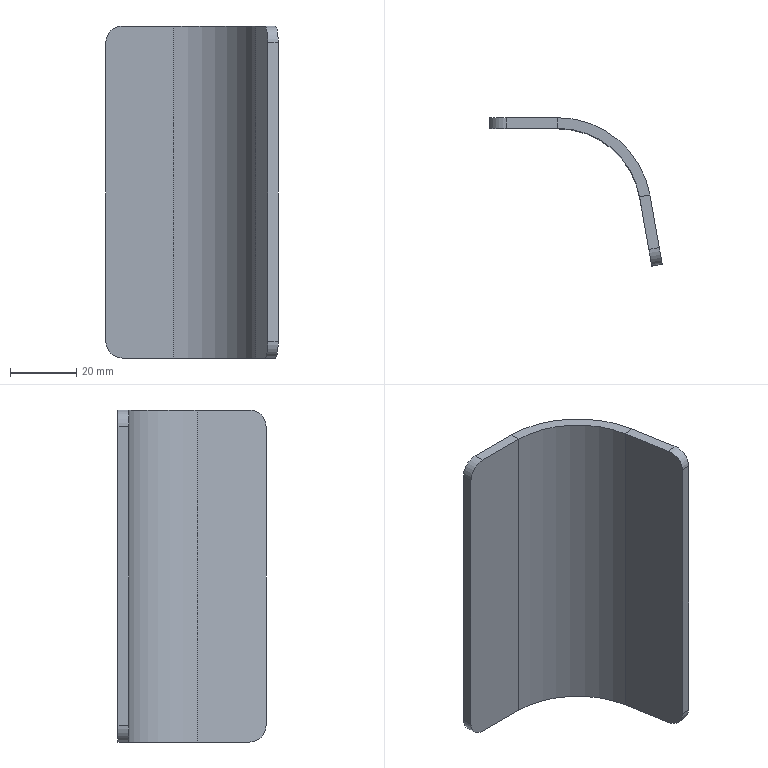Part | SolidWorks | features Fillet 1, FlatPattern 1, SMBaseFlange 1, SheetMetal 1 | 1 solid | 18 faces | box 51.9 x 44.589 x 100 mm | volume 25102 mm3 | plane 12 | cylinder 6 | commonest cylinder face diameters 10 x4 50 x1 56.4 x1
STEP:
#1=CARTESIAN_POINT('',(4.116,-23.293,50.));
#2=VERTEX_POINT('',#1);
#3=CARTESIAN_POINT('',(0.9645,-23.85,50.));
#4=VERTEX_POINT('',#3);
#5=CARTESIAN_POINT('',(4.116,-23.293,50.));
#6=DIRECTION('',(-0.9847,-0.174,0.));
#7=VECTOR('',#6,1000.);
#8=LINE('',#5,#7);
#9=EDGE_CURVE('',#2,#4,#8,.T.);
#10=ORIENTED_EDGE('',*,*,#9,.F.);
#11=CARTESIAN_POINT('',(-23.654,0.,50.));
#12=VERTEX_POINT('',#11);
#13=CARTESIAN_POINT('',(-23.654,-28.2,50.));
#14=DIRECTION('',(0.,0.,-1.));
#15=DIRECTION('',(1.,0.,0.));
#16=AXIS2_PLACEMENT_3D('',#13,#14,#15);
#17=CIRCLE('',#16,28.2);
#18=EDGE_CURVE('',#12,#2,#17,.T.);
#19=ORIENTED_EDGE('',*,*,#18,.F.);
#20=CARTESIAN_POINT('',(-23.654,-3.2,50.));
#21=VERTEX_POINT('',#20);
#22=CARTESIAN_POINT('',(-23.654,-3.2,50.));
#23=DIRECTION('',(0.,1.,0.));
#24=VECTOR('',#23,1000.);
#25=LINE('',#22,#24);
#26=EDGE_CURVE('',#21,#12,#25,.T.);
#27=ORIENTED_EDGE('',*,*,#26,.F.);
#28=CARTESIAN_POINT('',(-23.654,-28.2,50.));
#29=DIRECTION('',(0.,0.,-1.));
#30=DIRECTION('',(1.,0.,0.));
#31=AXIS2_PLACEMENT_3D('',#28,#29,#30);
#32=CIRCLE('',#31,25.);
#33=EDGE_CURVE('',#21,#4,#32,.T.);
#34=ORIENTED_EDGE('',*,*,#33,.T.);
#35=EDGE_LOOP('',(#10,#19,#27,#34));
#36=FACE_OUTER_BOUND('',#35,.T.);
#37=CARTESIAN_POINT('',(4.116,-23.293,50.));
#38=DIRECTION('',(0.,0.,1.));
#39=DIRECTION('',(1.,0.,0.));
#40=AXIS2_PLACEMENT_3D('',#37,#38,#39);
#41=PLANE('',#40);
#42=ADVANCED_FACE('',(#36),#41,.T.);
#43=CARTESIAN_POINT('',(3.759,-39.666,50.));
#44=VERTEX_POINT('',#43);
#45=CARTESIAN_POINT('',(-3.151,-0.5568,50.));
#46=DIRECTION('',(0.174,-0.9847,0.));
#47=VECTOR('',#46,1000.);
#48=LINE('',#45,#47);
#49=EDGE_CURVE('',#4,#44,#48,.T.);
#50=ORIENTED_EDGE('',*,*,#49,.T.);
#51=CARTESIAN_POINT('',(6.91,-39.109,50.));
#52=VERTEX_POINT('',#51);
#53=CARTESIAN_POINT('',(-16.576,-43.259,50.));
#54=DIRECTION('',(0.9847,0.174,0.));
#55=VECTOR('',#54,1000.);
#56=LINE('',#53,#55);
#57=EDGE_CURVE('',#44,#52,#56,.T.);
#58=ORIENTED_EDGE('',*,*,#57,.T.);
#59=CARTESIAN_POINT('',(0.,0.,50.));
#60=DIRECTION('',(0.174,-0.9847,0.));
#61=VECTOR('',#60,1000.);
#62=LINE('',#59,#61);
#63=EDGE_CURVE('',#2,#52,#62,.T.);
#64=ORIENTED_EDGE('',*,*,#63,.F.);
#65=ORIENTED_EDGE('',*,*,#9,.T.);
#66=EDGE_LOOP('',(#50,#58,#64,#65));
#67=FACE_OUTER_BOUND('',#66,.T.);
#68=CARTESIAN_POINT('',(-23.654,-3.2,50.));
#69=DIRECTION('',(0.,0.,1.));
#70=DIRECTION('',(1.,0.,0.));
#71=AXIS2_PLACEMENT_3D('',#68,#69,#70);
#72=PLANE('',#71);
#73=ADVANCED_FACE('',(#67),#72,.T.);
#74=CARTESIAN_POINT('',(-23.654,0.,-50.));
#75=VERTEX_POINT('',#74);
#76=CARTESIAN_POINT('',(-23.654,-3.2,-50.));
#77=VERTEX_POINT('',#76);
#78=CARTESIAN_POINT('',(-23.654,0.,-50.));
#79=DIRECTION('',(0.,-1.,0.));
#80=VECTOR('',#79,1000.);
#81=LINE('',#78,#80);
#82=EDGE_CURVE('',#75,#77,#81,.T.);
#83=ORIENTED_EDGE('',*,*,#82,.F.);
#84=CARTESIAN_POINT('',(4.116,-23.293,-50.));
#85=VERTEX_POINT('',#84);
#86=CARTESIAN_POINT('',(-23.654,-28.2,-50.));
#87=DIRECTION('',(0.,0.,-1.));
#88=DIRECTION('',(1.,0.,0.));
#89=AXIS2_PLACEMENT_3D('',#86,#87,#88);
#90=CIRCLE('',#89,28.2);
#91=EDGE_CURVE('',#75,#85,#90,.T.);
#92=ORIENTED_EDGE('',*,*,#91,.T.);
#93=CARTESIAN_POINT('',(0.9645,-23.85,-50.));
#94=VERTEX_POINT('',#93);
#95=CARTESIAN_POINT('',(0.9645,-23.85,-50.));
#96=DIRECTION('',(0.9847,0.174,0.));
#97=VECTOR('',#96,1000.);
#98=LINE('',#95,#97);
#99=EDGE_CURVE('',#94,#85,#98,.T.);
#100=ORIENTED_EDGE('',*,*,#99,.F.);
#101=CARTESIAN_POINT('',(-23.654,-28.2,-50.));
#102=DIRECTION('',(0.,0.,-1.));
#103=DIRECTION('',(1.,0.,0.));
#104=AXIS2_PLACEMENT_3D('',#101,#102,#103);
#105=CIRCLE('',#104,25.);
#106=EDGE_CURVE('',#77,#94,#105,.T.);
#107=ORIENTED_EDGE('',*,*,#106,.F.);
#108=EDGE_LOOP('',(#83,#92,#100,#107));
#109=FACE_OUTER_BOUND('',#108,.T.);
#110=CARTESIAN_POINT('',(-23.654,0.,-50.));
#111=DIRECTION('',(0.,0.,-1.));
#112=DIRECTION('',(-1.,0.,0.));
#113=AXIS2_PLACEMENT_3D('',#110,#111,#112);
#114=PLANE('',#113);
#115=ADVANCED_FACE('',(#109),#114,.T.);
#116=CARTESIAN_POINT('',(-39.12,-3.2,-50.));
#117=VERTEX_POINT('',#116);
#118=CARTESIAN_POINT('',(0.,-3.2,-50.));
#119=DIRECTION('',(1.,0.,0.));
#120=VECTOR('',#119,1000.);
#121=LINE('',#118,#120);
#122=EDGE_CURVE('',#117,#77,#121,.T.);
#123=ORIENTED_EDGE('',*,*,#122,.F.);
#124=CARTESIAN_POINT('',(-39.12,0.,-50.));
#125=VERTEX_POINT('',#124);
#126=CARTESIAN_POINT('',(-39.12,-23.85,-50.));
#127=DIRECTION('',(0.,1.,0.));
#128=VECTOR('',#127,1000.);
#129=LINE('',#126,#128);
#130=EDGE_CURVE('',#117,#125,#129,.T.);
#131=ORIENTED_EDGE('',*,*,#130,.T.);
#132=CARTESIAN_POINT('',(0.,0.,-50.));
#133=DIRECTION('',(1.,0.,0.));
#134=VECTOR('',#133,1000.);
#135=LINE('',#132,#134);
#136=EDGE_CURVE('',#125,#75,#135,.T.);
#137=ORIENTED_EDGE('',*,*,#136,.T.);
#138=ORIENTED_EDGE('',*,*,#82,.T.);
#139=EDGE_LOOP('',(#123,#131,#137,#138));
#140=FACE_OUTER_BOUND('',#139,.T.);
#141=CARTESIAN_POINT('',(0.9645,-23.85,-50.));
#142=DIRECTION('',(0.,0.,-1.));
#143=DIRECTION('',(-1.,0.,0.));
#144=AXIS2_PLACEMENT_3D('',#141,#142,#143);
#145=PLANE('',#144);
#146=ADVANCED_FACE('',(#140),#145,.T.);
#147=CARTESIAN_POINT('',(4.629,-44.589,45.));
#148=VERTEX_POINT('',#147);
#149=CARTESIAN_POINT('',(4.629,-44.589,-45.));
#150=VERTEX_POINT('',#149);
#151=CARTESIAN_POINT('',(4.629,-44.589,50.));
#152=DIRECTION('',(0.,0.,-1.));
#153=VECTOR('',#152,1000.);
#154=LINE('',#151,#153);
#155=EDGE_CURVE('',#148,#150,#154,.T.);
#156=ORIENTED_EDGE('',*,*,#155,.F.);
#157=CARTESIAN_POINT('',(3.759,-39.666,45.));
#158=DIRECTION('',(-0.9847,-0.174,0.));
#159=DIRECTION('',(-0.174,0.9847,0.));
#160=AXIS2_PLACEMENT_3D('',#157,#158,#159);
#161=CIRCLE('',#160,5.);
#162=EDGE_CURVE('',#148,#44,#161,.T.);
#163=ORIENTED_EDGE('',*,*,#162,.T.);
#164=ORIENTED_EDGE('',*,*,#49,.F.);
#165=CARTESIAN_POINT('',(0.9645,-23.85,50.));
#166=DIRECTION('',(0.,0.,-1.));
#167=VECTOR('',#166,1000.);
#168=LINE('',#165,#167);
#169=EDGE_CURVE('',#4,#94,#168,.T.);
#170=ORIENTED_EDGE('',*,*,#169,.T.);
#171=CARTESIAN_POINT('',(3.759,-39.666,-50.));
#172=VERTEX_POINT('',#171);
#173=CARTESIAN_POINT('',(-3.151,-0.5568,-50.));
#174=DIRECTION('',(0.174,-0.9847,0.));
#175=VECTOR('',#174,1000.);
#176=LINE('',#173,#175);
#177=EDGE_CURVE('',#94,#172,#176,.T.);
#178=ORIENTED_EDGE('',*,*,#177,.T.);
#179=CARTESIAN_POINT('',(3.759,-39.666,-45.));
#180=DIRECTION('',(-0.9847,-0.174,0.));
#181=DIRECTION('',(-0.174,0.9847,0.));
#182=AXIS2_PLACEMENT_3D('',#179,#180,#181);
#183=CIRCLE('',#182,5.);
#184=EDGE_CURVE('',#172,#150,#183,.T.);
#185=ORIENTED_EDGE('',*,*,#184,.T.);
#186=EDGE_LOOP('',(#156,#163,#164,#170,#178,#185));
#187=FACE_OUTER_BOUND('',#186,.T.);
#188=CARTESIAN_POINT('',(-3.151,-0.5568,50.));
#189=DIRECTION('',(0.9847,0.174,0.));
#190=DIRECTION('',(-0.174,0.9847,0.));
#191=AXIS2_PLACEMENT_3D('',#188,#189,#190);
#192=PLANE('',#191);
#193=ADVANCED_FACE('',(#187),#192,.F.);
#194=CARTESIAN_POINT('',(7.78,-44.033,45.));
#195=VERTEX_POINT('',#194);
#196=CARTESIAN_POINT('',(7.78,-44.033,-45.));
#197=VERTEX_POINT('',#196);
#198=CARTESIAN_POINT('',(7.78,-44.033,50.));
#199=DIRECTION('',(0.,0.,-1.));
#200=VECTOR('',#199,1000.);
#201=LINE('',#198,#200);
#202=EDGE_CURVE('',#195,#197,#201,.T.);
#203=ORIENTED_EDGE('',*,*,#202,.F.);
#204=CARTESIAN_POINT('',(7.78,-44.033,45.));
#205=DIRECTION('',(-0.9847,-0.174,0.));
#206=VECTOR('',#205,1000.);
#207=LINE('',#204,#206);
#208=EDGE_CURVE('',#195,#148,#207,.T.);
#209=ORIENTED_EDGE('',*,*,#208,.T.);
#210=ORIENTED_EDGE('',*,*,#155,.T.);
#211=CARTESIAN_POINT('',(7.78,-44.033,-45.));
#212=DIRECTION('',(0.9847,0.174,0.));
#213=VECTOR('',#212,1000.);
#214=LINE('',#211,#213);
#215=EDGE_CURVE('',#150,#197,#214,.T.);
#216=ORIENTED_EDGE('',*,*,#215,.T.);
#217=EDGE_LOOP('',(#203,#209,#210,#216));
#218=FACE_OUTER_BOUND('',#217,.T.);
#219=CARTESIAN_POINT('',(7.78,-44.033,50.));
#220=DIRECTION('',(0.174,-0.9847,0.));
#221=DIRECTION('',(0.9847,0.174,0.));
#222=AXIS2_PLACEMENT_3D('',#219,#220,#221);
#223=PLANE('',#222);
#224=ADVANCED_FACE('',(#218),#223,.T.);
#225=ORIENTED_EDGE('',*,*,#63,.T.);
#226=CARTESIAN_POINT('',(6.91,-39.109,45.));
#227=DIRECTION('',(0.9847,0.174,0.));
#228=DIRECTION('',(-0.174,0.9847,0.));
#229=AXIS2_PLACEMENT_3D('',#226,#227,#228);
#230=CIRCLE('',#229,5.);
#231=EDGE_CURVE('',#52,#195,#230,.T.);
#232=ORIENTED_EDGE('',*,*,#231,.T.);
#233=ORIENTED_EDGE('',*,*,#202,.T.);
#234=CARTESIAN_POINT('',(6.91,-39.109,-50.));
#235=VERTEX_POINT('',#234);
#236=CARTESIAN_POINT('',(6.91,-39.109,-45.));
#237=DIRECTION('',(0.9847,0.174,0.));
#238=DIRECTION('',(-0.174,0.9847,0.));
#239=AXIS2_PLACEMENT_3D('',#236,#237,#238);
#240=CIRCLE('',#239,5.);
#241=EDGE_CURVE('',#197,#235,#240,.T.);
#242=ORIENTED_EDGE('',*,*,#241,.T.);
#243=CARTESIAN_POINT('',(0.,0.,-50.));
#244=DIRECTION('',(0.174,-0.9847,0.));
#245=VECTOR('',#244,1000.);
#246=LINE('',#243,#245);
#247=EDGE_CURVE('',#85,#235,#246,.T.);
#248=ORIENTED_EDGE('',*,*,#247,.F.);
#249=CARTESIAN_POINT('',(4.116,-23.293,50.));
#250=DIRECTION('',(0.,0.,-1.));
#251=VECTOR('',#250,1000.);
#252=LINE('',#249,#251);
#253=EDGE_CURVE('',#2,#85,#252,.T.);
#254=ORIENTED_EDGE('',*,*,#253,.F.);
#255=EDGE_LOOP('',(#225,#232,#233,#242,#248,#254));
#256=FACE_OUTER_BOUND('',#255,.T.);
#257=CARTESIAN_POINT('',(0.,0.,50.));
#258=DIRECTION('',(0.9847,0.174,0.));
#259=DIRECTION('',(-0.174,0.9847,0.));
#260=AXIS2_PLACEMENT_3D('',#257,#258,#259);
#261=PLANE('',#260);
#262=ADVANCED_FACE('',(#256),#261,.T.);
#263=ORIENTED_EDGE('',*,*,#91,.F.);
#264=CARTESIAN_POINT('',(-23.654,0.,50.));
#265=DIRECTION('',(0.,0.,-1.));
#266=VECTOR('',#265,1000.);
#267=LINE('',#264,#266);
#268=EDGE_CURVE('',#12,#75,#267,.T.);
#269=ORIENTED_EDGE('',*,*,#268,.F.);
#270=ORIENTED_EDGE('',*,*,#18,.T.);
#271=ORIENTED_EDGE('',*,*,#253,.T.);
#272=EDGE_LOOP('',(#263,#269,#270,#271));
#273=FACE_OUTER_BOUND('',#272,.T.);
#274=CARTESIAN_POINT('',(-23.654,-28.2,50.));
#275=DIRECTION('',(0.,0.,-1.));
#276=DIRECTION('',(-1.,0.,0.));
#277=AXIS2_PLACEMENT_3D('',#274,#275,#276);
#278=CYLINDRICAL_SURFACE('',#277,28.2);
#279=ADVANCED_FACE('',(#273),#278,.T.);
#280=ORIENTED_EDGE('',*,*,#136,.F.);
#281=CARTESIAN_POINT('',(-44.12,0.,-45.));
#282=VERTEX_POINT('',#281);
#283=CARTESIAN_POINT('',(-39.12,0.,-45.));
#284=DIRECTION('',(0.,1.,0.));
#285=DIRECTION('',(-1.,0.,0.));
#286=AXIS2_PLACEMENT_3D('',#283,#284,#285);
#287=CIRCLE('',#286,5.);
#288=EDGE_CURVE('',#125,#282,#287,.T.);
#289=ORIENTED_EDGE('',*,*,#288,.T.);
#290=CARTESIAN_POINT('',(-44.12,0.,45.));
#291=VERTEX_POINT('',#290);
#292=CARTESIAN_POINT('',(-44.12,0.,50.));
#293=DIRECTION('',(0.,0.,-1.));
#294=VECTOR('',#293,1000.);
#295=LINE('',#292,#294);
#296=EDGE_CURVE('',#291,#282,#295,.T.);
#297=ORIENTED_EDGE('',*,*,#296,.F.);
#298=CARTESIAN_POINT('',(-39.12,0.,50.));
#299=VERTEX_POINT('',#298);
#300=CARTESIAN_POINT('',(-39.12,0.,45.));
#301=DIRECTION('',(0.,1.,0.));
#302=DIRECTION('',(-1.,0.,0.));
#303=AXIS2_PLACEMENT_3D('',#300,#301,#302);
#304=CIRCLE('',#303,5.);
#305=EDGE_CURVE('',#291,#299,#304,.T.);
#306=ORIENTED_EDGE('',*,*,#305,.T.);
#307=CARTESIAN_POINT('',(0.,0.,50.));
#308=DIRECTION('',(1.,0.,0.));
#309=VECTOR('',#308,1000.);
#310=LINE('',#307,#309);
#311=EDGE_CURVE('',#299,#12,#310,.T.);
#312=ORIENTED_EDGE('',*,*,#311,.T.);
#313=ORIENTED_EDGE('',*,*,#268,.T.);
#314=EDGE_LOOP('',(#280,#289,#297,#306,#312,#313));
#315=FACE_OUTER_BOUND('',#314,.T.);
#316=CARTESIAN_POINT('',(0.,0.,50.));
#317=DIRECTION('',(0.,1.,0.));
#318=DIRECTION('',(-1.,0.,0.));
#319=AXIS2_PLACEMENT_3D('',#316,#317,#318);
#320=PLANE('',#319);
#321=ADVANCED_FACE('',(#315),#320,.T.);
#322=ORIENTED_EDGE('',*,*,#296,.T.);
#323=CARTESIAN_POINT('',(-44.12,-3.2,-45.));
#324=VERTEX_POINT('',#323);
#325=CARTESIAN_POINT('',(-44.12,-3.2,-45.));
#326=DIRECTION('',(0.,-1.,0.));
#327=VECTOR('',#326,1000.);
#328=LINE('',#325,#327);
#329=EDGE_CURVE('',#282,#324,#328,.T.);
#330=ORIENTED_EDGE('',*,*,#329,.T.);
#331=CARTESIAN_POINT('',(-44.12,-3.2,45.));
#332=VERTEX_POINT('',#331);
#333=CARTESIAN_POINT('',(-44.12,-3.2,50.));
#334=DIRECTION('',(0.,0.,-1.));
#335=VECTOR('',#334,1000.);
#336=LINE('',#333,#335);
#337=EDGE_CURVE('',#332,#324,#336,.T.);
#338=ORIENTED_EDGE('',*,*,#337,.F.);
#339=CARTESIAN_POINT('',(-44.12,-3.2,45.));
#340=DIRECTION('',(0.,1.,0.));
#341=VECTOR('',#340,1000.);
#342=LINE('',#339,#341);
#343=EDGE_CURVE('',#332,#291,#342,.T.);
#344=ORIENTED_EDGE('',*,*,#343,.T.);
#345=EDGE_LOOP('',(#322,#330,#338,#344));
#346=FACE_OUTER_BOUND('',#345,.T.);
#347=CARTESIAN_POINT('',(-44.12,-3.2,50.));
#348=DIRECTION('',(-1.,0.,0.));
#349=DIRECTION('',(0.,0.,1.));
#350=AXIS2_PLACEMENT_3D('',#347,#348,#349);
#351=PLANE('',#350);
#352=ADVANCED_FACE('',(#346),#351,.T.);
#353=ORIENTED_EDGE('',*,*,#337,.T.);
#354=CARTESIAN_POINT('',(-39.12,-3.2,-45.));
#355=DIRECTION('',(0.,-1.,0.));
#356=DIRECTION('',(-1.,0.,0.));
#357=AXIS2_PLACEMENT_3D('',#354,#355,#356);
#358=CIRCLE('',#357,5.);
#359=EDGE_CURVE('',#324,#117,#358,.T.);
#360=ORIENTED_EDGE('',*,*,#359,.T.);
#361=ORIENTED_EDGE('',*,*,#122,.T.);
#362=CARTESIAN_POINT('',(-23.654,-3.2,50.));
#363=DIRECTION('',(0.,0.,-1.));
#364=VECTOR('',#363,1000.);
#365=LINE('',#362,#364);
#366=EDGE_CURVE('',#21,#77,#365,.T.);
#367=ORIENTED_EDGE('',*,*,#366,.F.);
#368=CARTESIAN_POINT('',(-39.12,-3.2,50.));
#369=VERTEX_POINT('',#368);
#370=CARTESIAN_POINT('',(0.,-3.2,50.));
#371=DIRECTION('',(1.,0.,0.));
#372=VECTOR('',#371,1000.);
#373=LINE('',#370,#372);
#374=EDGE_CURVE('',#369,#21,#373,.T.);
#375=ORIENTED_EDGE('',*,*,#374,.F.);
#376=CARTESIAN_POINT('',(-39.12,-3.2,45.));
#377=DIRECTION('',(0.,-1.,0.));
#378=DIRECTION('',(-1.,0.,0.));
#379=AXIS2_PLACEMENT_3D('',#376,#377,#378);
#380=CIRCLE('',#379,5.);
#381=EDGE_CURVE('',#369,#332,#380,.T.);
#382=ORIENTED_EDGE('',*,*,#381,.T.);
#383=EDGE_LOOP('',(#353,#360,#361,#367,#375,#382));
#384=FACE_OUTER_BOUND('',#383,.T.);
#385=CARTESIAN_POINT('',(0.,-3.2,50.));
#386=DIRECTION('',(0.,1.,0.));
#387=DIRECTION('',(-1.,0.,0.));
#388=AXIS2_PLACEMENT_3D('',#385,#386,#387);
#389=PLANE('',#388);
#390=ADVANCED_FACE('',(#384),#389,.F.);
#391=ORIENTED_EDGE('',*,*,#106,.T.);
#392=ORIENTED_EDGE('',*,*,#169,.F.);
#393=ORIENTED_EDGE('',*,*,#33,.F.);
#394=ORIENTED_EDGE('',*,*,#366,.T.);
#395=EDGE_LOOP('',(#391,#392,#393,#394));
#396=FACE_OUTER_BOUND('',#395,.T.);
#397=CARTESIAN_POINT('',(-23.654,-28.2,50.));
#398=DIRECTION('',(0.,0.,-1.));
#399=DIRECTION('',(-1.,0.,0.));
#400=AXIS2_PLACEMENT_3D('',#397,#398,#399);
#401=CYLINDRICAL_SURFACE('',#400,25.);
#402=ADVANCED_FACE('',(#396),#401,.F.);
#403=ORIENTED_EDGE('',*,*,#311,.F.);
#404=CARTESIAN_POINT('',(-39.12,-28.2,50.));
#405=DIRECTION('',(0.,-1.,0.));
#406=VECTOR('',#405,1000.);
#407=LINE('',#404,#406);
#408=EDGE_CURVE('',#299,#369,#407,.T.);
#409=ORIENTED_EDGE('',*,*,#408,.T.);
#410=ORIENTED_EDGE('',*,*,#374,.T.);
#411=ORIENTED_EDGE('',*,*,#26,.T.);
#412=EDGE_LOOP('',(#403,#409,#410,#411));
#413=FACE_OUTER_BOUND('',#412,.T.);
#414=CARTESIAN_POINT('',(-23.654,-28.2,50.));
#415=DIRECTION('',(0.,0.,1.));
#416=DIRECTION('',(1.,0.,0.));
#417=AXIS2_PLACEMENT_3D('',#414,#415,#416);
#418=PLANE('',#417);
#419=ADVANCED_FACE('',(#413),#418,.T.);
#420=ORIENTED_EDGE('',*,*,#247,.T.);
#421=CARTESIAN_POINT('',(3.759,-39.666,-50.));
#422=DIRECTION('',(-0.9847,-0.174,0.));
#423=VECTOR('',#422,1000.);
#424=LINE('',#421,#423);
#425=EDGE_CURVE('',#235,#172,#424,.T.);
#426=ORIENTED_EDGE('',*,*,#425,.T.);
#427=ORIENTED_EDGE('',*,*,#177,.F.);
#428=ORIENTED_EDGE('',*,*,#99,.T.);
#429=EDGE_LOOP('',(#420,#426,#427,#428));
#430=FACE_OUTER_BOUND('',#429,.T.);
#431=CARTESIAN_POINT('',(-23.654,-28.2,-50.));
#432=DIRECTION('',(0.,0.,1.));
#433=DIRECTION('',(1.,0.,0.));
#434=AXIS2_PLACEMENT_3D('',#431,#432,#433);
#435=PLANE('',#434);
#436=ADVANCED_FACE('',(#430),#435,.F.);
#437=ORIENTED_EDGE('',*,*,#359,.F.);
#438=ORIENTED_EDGE('',*,*,#329,.F.);
#439=ORIENTED_EDGE('',*,*,#288,.F.);
#440=ORIENTED_EDGE('',*,*,#130,.F.);
#441=EDGE_LOOP('',(#437,#438,#439,#440));
#442=FACE_OUTER_BOUND('',#441,.T.);
#443=CARTESIAN_POINT('',(-39.12,-23.85,-45.));
#444=DIRECTION('',(0.,1.,0.));
#445=DIRECTION('',(0.,0.,1.));
#446=AXIS2_PLACEMENT_3D('',#443,#444,#445);
#447=CYLINDRICAL_SURFACE('',#446,5.);
#448=ADVANCED_FACE('',(#442),#447,.T.);
#449=ORIENTED_EDGE('',*,*,#381,.F.);
#450=ORIENTED_EDGE('',*,*,#408,.F.);
#451=ORIENTED_EDGE('',*,*,#305,.F.);
#452=ORIENTED_EDGE('',*,*,#343,.F.);
#453=EDGE_LOOP('',(#449,#450,#451,#452));
#454=FACE_OUTER_BOUND('',#453,.T.);
#455=CARTESIAN_POINT('',(-39.12,-3.2,45.));
#456=DIRECTION('',(0.,1.,0.));
#457=DIRECTION('',(0.,0.,1.));
#458=AXIS2_PLACEMENT_3D('',#455,#456,#457);
#459=CYLINDRICAL_SURFACE('',#458,5.);
#460=ADVANCED_FACE('',(#454),#459,.T.);
#461=ORIENTED_EDGE('',*,*,#231,.F.);
#462=ORIENTED_EDGE('',*,*,#57,.F.);
#463=ORIENTED_EDGE('',*,*,#162,.F.);
#464=ORIENTED_EDGE('',*,*,#208,.F.);
#465=EDGE_LOOP('',(#461,#462,#463,#464));
#466=FACE_OUTER_BOUND('',#465,.T.);
#467=CARTESIAN_POINT('',(6.91,-39.109,45.));
#468=DIRECTION('',(-0.9847,-0.174,0.));
#469=DIRECTION('',(0.174,-0.9847,0.));
#470=AXIS2_PLACEMENT_3D('',#467,#468,#469);
#471=CYLINDRICAL_SURFACE('',#470,5.);
#472=ADVANCED_FACE('',(#466),#471,.T.);
#473=ORIENTED_EDGE('',*,*,#241,.F.);
#474=ORIENTED_EDGE('',*,*,#215,.F.);
#475=ORIENTED_EDGE('',*,*,#184,.F.);
#476=ORIENTED_EDGE('',*,*,#425,.F.);
#477=EDGE_LOOP('',(#473,#474,#475,#476));
#478=FACE_OUTER_BOUND('',#477,.T.);
#479=CARTESIAN_POINT('',(-20.86,-44.016,-45.));
#480=DIRECTION('',(0.9847,0.174,0.));
#481=DIRECTION('',(-0.174,0.9847,0.));
#482=AXIS2_PLACEMENT_3D('',#479,#480,#481);
#483=CYLINDRICAL_SURFACE('',#482,5.);
#484=ADVANCED_FACE('',(#478),#483,.T.);
#485=CLOSED_SHELL('',(#42,#73,#115,#146,#193,#224,#262,#279,#321,#352,#390,#402,#419,#436,#448,#460,#472,#484));
#486=MANIFOLD_SOLID_BREP('',#485);
#487=CARTESIAN_POINT('',(0.,0.,0.));
#488=DIRECTION('',(0.,0.,1.));
#489=DIRECTION('',(1.,0.,0.));
#490=AXIS2_PLACEMENT_3D('',#487,#488,#489);
#491=(LENGTH_UNIT()NAMED_UNIT(*)SI_UNIT(.MILLI.,.METRE.));
#492=UNCERTAINTY_MEASURE_WITH_UNIT(LENGTH_MEASURE(0.00001),#491,'','');
#493=(NAMED_UNIT(*)PLANE_ANGLE_UNIT()SI_UNIT($,.RADIAN.));
#494=(NAMED_UNIT(*)SI_UNIT($,.STERADIAN.)SOLID_ANGLE_UNIT());
#495=(GEOMETRIC_REPRESENTATION_CONTEXT(3)GLOBAL_UNCERTAINTY_ASSIGNED_CONTEXT((#492))GLOBAL_UNIT_ASSIGNED_CONTEXT((#491,#493,#494))REPRESENTATION_CONTEXT('',''));
#496=ADVANCED_BREP_SHAPE_REPRESENTATION('',(#486,#490),#495);